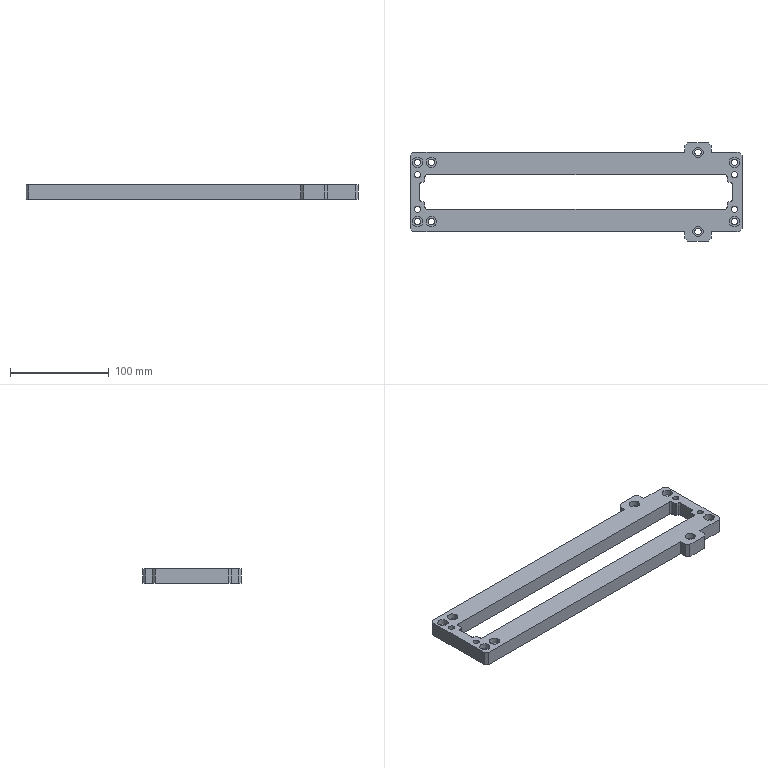Part | STEP file | Tube feed_id814_x_t | 1 solid | 82 faces | box 336 x 100 x 15 mm | volume 239179 mm3 | plane 50 | cylinder 32 | commonest cylinder face diameters 4 x8 6.5 x8 10.5 x8 6 x4 12 x4